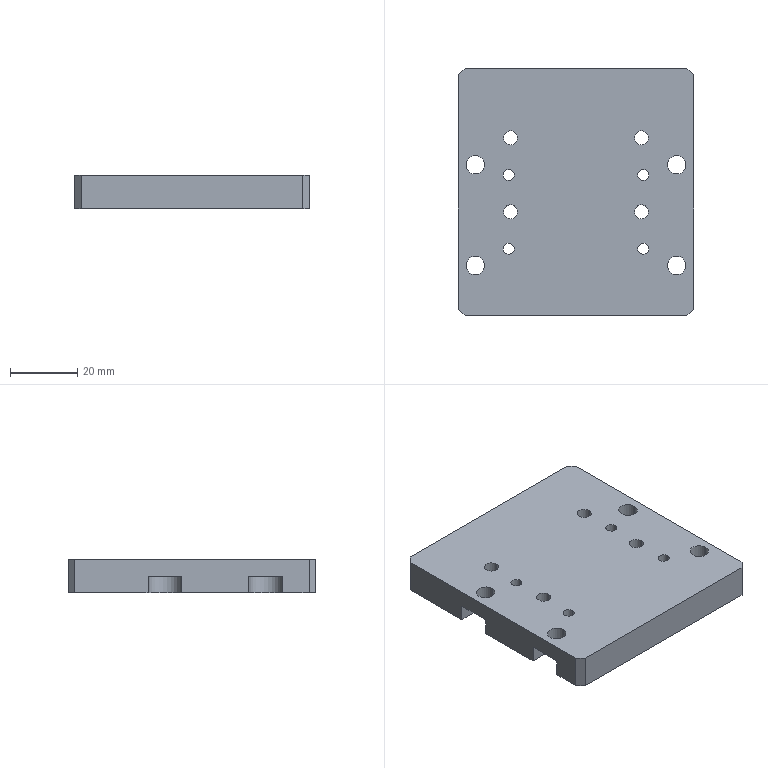Part | STEP file | 04-02-04 small base plate C | 1 solid | 55 faces | box 70 x 73.8 x 10 mm | volume 48282 mm3 | cylinder 32 | plane 23 | commonest cylinder face diameters 3.3 x8 4.2 x8 5.5 x8 10 x6 6 x2